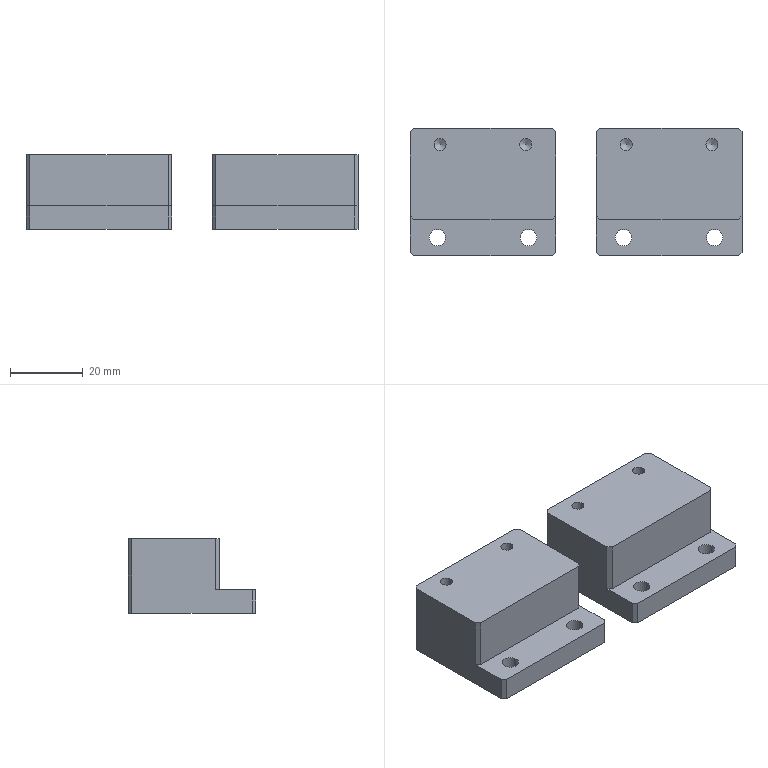Part | NX | 2 solids | 40 faces | box 91 x 35 x 20.5 mm | volume 45300 mm3 | plane 28 | cylinder 8 | cone 4 | commonest cylinder face diameters 3.3 x4 4.5 x4
STEP:
#1=CARTESIAN_POINT('',(-31.,-6.5,-3.75));
#2=VERTEX_POINT('',#1);
#3=CARTESIAN_POINT('',(-32.,-7.5,-3.75));
#4=VERTEX_POINT('',#3);
#5=CARTESIAN_POINT('',(-56.5,-32.,-3.75));
#6=DIRECTION('',(-0.7071,-0.7071,0.));
#7=VECTOR('',#6,1000.);
#8=LINE('',#5,#7);
#9=EDGE_CURVE('',#2,#4,#8,.T.);
#10=ORIENTED_EDGE('',*,*,#9,.F.);
#11=CARTESIAN_POINT('',(-31.,-6.5,10.25));
#12=VERTEX_POINT('',#11);
#13=CARTESIAN_POINT('',(-31.,-6.5,10.25));
#14=DIRECTION('',(0.,0.,-1.));
#15=VECTOR('',#14,1000.);
#16=LINE('',#13,#15);
#17=EDGE_CURVE('',#12,#2,#16,.T.);
#18=ORIENTED_EDGE('',*,*,#17,.F.);
#19=CARTESIAN_POINT('',(-32.,-7.5,10.25));
#20=VERTEX_POINT('',#19);
#21=CARTESIAN_POINT('',(-37.75,-13.25,10.25));
#22=DIRECTION('',(0.7071,0.7071,0.));
#23=VECTOR('',#22,1000.);
#24=LINE('',#21,#23);
#25=EDGE_CURVE('',#20,#12,#24,.T.);
#26=ORIENTED_EDGE('',*,*,#25,.F.);
#27=CARTESIAN_POINT('',(-32.,-7.5,10.25));
#28=DIRECTION('',(0.,0.,1.));
#29=VECTOR('',#28,1000.);
#30=LINE('',#27,#29);
#31=EDGE_CURVE('',#4,#20,#30,.T.);
#32=ORIENTED_EDGE('',*,*,#31,.F.);
#33=EDGE_LOOP('',(#10,#18,#26,#32));
#34=FACE_BOUND('',#33,.T.);
#35=CARTESIAN_POINT('',(-32.,-7.5,10.25));
#36=DIRECTION('',(-0.7071,0.7071,0.));
#37=DIRECTION('',(0.,0.,1.));
#38=AXIS2_PLACEMENT_3D('',#35,#36,#37);
#39=PLANE('',#38);
#40=ADVANCED_FACE('',(#34),#39,.F.);
#41=CARTESIAN_POINT('',(-31.,16.5,10.25));
#42=VERTEX_POINT('',#41);
#43=CARTESIAN_POINT('',(-32.,17.5,10.25));
#44=VERTEX_POINT('',#43);
#45=CARTESIAN_POINT('',(-32.75,18.25,10.25));
#46=DIRECTION('',(-0.7071,0.7071,0.));
#47=VECTOR('',#46,1000.);
#48=LINE('',#45,#47);
#49=EDGE_CURVE('',#42,#44,#48,.T.);
#50=ORIENTED_EDGE('',*,*,#49,.F.);
#51=CARTESIAN_POINT('',(-31.,16.5,-10.25));
#52=VERTEX_POINT('',#51);
#53=CARTESIAN_POINT('',(-31.,16.5,10.25));
#54=DIRECTION('',(0.,0.,1.));
#55=VECTOR('',#54,1000.);
#56=LINE('',#53,#55);
#57=EDGE_CURVE('',#52,#42,#56,.T.);
#58=ORIENTED_EDGE('',*,*,#57,.F.);
#59=CARTESIAN_POINT('',(-32.,17.5,-10.25));
#60=VERTEX_POINT('',#59);
#61=CARTESIAN_POINT('',(-32.,17.5,-10.25));
#62=DIRECTION('',(0.7071,-0.7071,0.));
#63=VECTOR('',#62,1000.);
#64=LINE('',#61,#63);
#65=EDGE_CURVE('',#60,#52,#64,.T.);
#66=ORIENTED_EDGE('',*,*,#65,.F.);
#67=CARTESIAN_POINT('',(-32.,17.5,10.25));
#68=DIRECTION('',(0.,0.,-1.));
#69=VECTOR('',#68,1000.);
#70=LINE('',#67,#69);
#71=EDGE_CURVE('',#44,#60,#70,.T.);
#72=ORIENTED_EDGE('',*,*,#71,.F.);
#73=EDGE_LOOP('',(#50,#58,#66,#72));
#74=FACE_BOUND('',#73,.T.);
#75=CARTESIAN_POINT('',(-32.,17.5,10.25));
#76=DIRECTION('',(-0.7071,-0.7071,0.));
#77=DIRECTION('',(0.,0.,-1.));
#78=AXIS2_PLACEMENT_3D('',#75,#76,#77);
#79=PLANE('',#78);
#80=ADVANCED_FACE('',(#74),#79,.F.);
#81=CARTESIAN_POINT('',(-70.,17.5,10.25));
#82=VERTEX_POINT('',#81);
#83=CARTESIAN_POINT('',(-71.,16.5,10.25));
#84=VERTEX_POINT('',#83);
#85=CARTESIAN_POINT('',(-69.25,18.25,10.25));
#86=DIRECTION('',(-0.7071,-0.7071,0.));
#87=VECTOR('',#86,1000.);
#88=LINE('',#85,#87);
#89=EDGE_CURVE('',#82,#84,#88,.T.);
#90=ORIENTED_EDGE('',*,*,#89,.F.);
#91=CARTESIAN_POINT('',(-70.,17.5,-10.25));
#92=VERTEX_POINT('',#91);
#93=CARTESIAN_POINT('',(-70.,17.5,10.25));
#94=DIRECTION('',(0.,0.,1.));
#95=VECTOR('',#94,1000.);
#96=LINE('',#93,#95);
#97=EDGE_CURVE('',#92,#82,#96,.T.);
#98=ORIENTED_EDGE('',*,*,#97,.F.);
#99=CARTESIAN_POINT('',(-71.,16.5,-10.25));
#100=VERTEX_POINT('',#99);
#101=CARTESIAN_POINT('',(-71.,16.5,-10.25));
#102=DIRECTION('',(0.7071,0.7071,0.));
#103=VECTOR('',#102,1000.);
#104=LINE('',#101,#103);
#105=EDGE_CURVE('',#100,#92,#104,.T.);
#106=ORIENTED_EDGE('',*,*,#105,.F.);
#107=CARTESIAN_POINT('',(-71.,16.5,10.25));
#108=DIRECTION('',(0.,0.,-1.));
#109=VECTOR('',#108,1000.);
#110=LINE('',#107,#109);
#111=EDGE_CURVE('',#84,#100,#110,.T.);
#112=ORIENTED_EDGE('',*,*,#111,.F.);
#113=EDGE_LOOP('',(#90,#98,#106,#112));
#114=FACE_BOUND('',#113,.T.);
#115=CARTESIAN_POINT('',(-71.,16.5,10.25));
#116=DIRECTION('',(0.7071,-0.7071,0.));
#117=DIRECTION('',(0.,0.,-1.));
#118=AXIS2_PLACEMENT_3D('',#115,#116,#117);
#119=PLANE('',#118);
#120=ADVANCED_FACE('',(#114),#119,.F.);
#121=CARTESIAN_POINT('',(-70.,-7.5,-3.75));
#122=VERTEX_POINT('',#121);
#123=CARTESIAN_POINT('',(-71.,-6.5,-3.75));
#124=VERTEX_POINT('',#123);
#125=CARTESIAN_POINT('',(-65.5,-12.,-3.75));
#126=DIRECTION('',(-0.7071,0.7071,0.));
#127=VECTOR('',#126,1000.);
#128=LINE('',#125,#127);
#129=EDGE_CURVE('',#122,#124,#128,.T.);
#130=ORIENTED_EDGE('',*,*,#129,.F.);
#131=CARTESIAN_POINT('',(-70.,-7.5,10.25));
#132=VERTEX_POINT('',#131);
#133=CARTESIAN_POINT('',(-70.,-7.5,10.25));
#134=DIRECTION('',(0.,0.,-1.));
#135=VECTOR('',#134,1000.);
#136=LINE('',#133,#135);
#137=EDGE_CURVE('',#132,#122,#136,.T.);
#138=ORIENTED_EDGE('',*,*,#137,.F.);
#139=CARTESIAN_POINT('',(-71.,-6.5,10.25));
#140=VERTEX_POINT('',#139);
#141=CARTESIAN_POINT('',(-64.25,-13.25,10.25));
#142=DIRECTION('',(0.7071,-0.7071,0.));
#143=VECTOR('',#142,1000.);
#144=LINE('',#141,#143);
#145=EDGE_CURVE('',#140,#132,#144,.T.);
#146=ORIENTED_EDGE('',*,*,#145,.F.);
#147=CARTESIAN_POINT('',(-71.,-6.5,10.25));
#148=DIRECTION('',(0.,0.,1.));
#149=VECTOR('',#148,1000.);
#150=LINE('',#147,#149);
#151=EDGE_CURVE('',#124,#140,#150,.T.);
#152=ORIENTED_EDGE('',*,*,#151,.F.);
#153=EDGE_LOOP('',(#130,#138,#146,#152));
#154=FACE_BOUND('',#153,.T.);
#155=CARTESIAN_POINT('',(-71.,-6.5,10.25));
#156=DIRECTION('',(0.7071,0.7071,0.));
#157=DIRECTION('',(0.,0.,1.));
#158=AXIS2_PLACEMENT_3D('',#155,#156,#157);
#159=PLANE('',#158);
#160=ADVANCED_FACE('',(#154),#159,.F.);
#161=CARTESIAN_POINT('',(-71.,-16.5,-3.75));
#162=VERTEX_POINT('',#161);
#163=CARTESIAN_POINT('',(-70.,-17.5,-3.75));
#164=VERTEX_POINT('',#163);
#165=CARTESIAN_POINT('',(-70.,-17.5,-3.75));
#166=DIRECTION('',(0.7071,-0.7071,0.));
#167=VECTOR('',#166,1000.);
#168=LINE('',#165,#167);
#169=EDGE_CURVE('',#162,#164,#168,.T.);
#170=ORIENTED_EDGE('',*,*,#169,.F.);
#171=CARTESIAN_POINT('',(-71.,-16.5,-10.25));
#172=VERTEX_POINT('',#171);
#173=CARTESIAN_POINT('',(-71.,-16.5,10.25));
#174=DIRECTION('',(0.,0.,1.));
#175=VECTOR('',#174,1000.);
#176=LINE('',#173,#175);
#177=EDGE_CURVE('',#172,#162,#176,.T.);
#178=ORIENTED_EDGE('',*,*,#177,.F.);
#179=CARTESIAN_POINT('',(-70.,-17.5,-10.25));
#180=VERTEX_POINT('',#179);
#181=CARTESIAN_POINT('',(-70.,-17.5,-10.25));
#182=DIRECTION('',(-0.7071,0.7071,0.));
#183=VECTOR('',#182,1000.);
#184=LINE('',#181,#183);
#185=EDGE_CURVE('',#180,#172,#184,.T.);
#186=ORIENTED_EDGE('',*,*,#185,.F.);
#187=CARTESIAN_POINT('',(-70.,-17.5,10.25));
#188=DIRECTION('',(0.,0.,-1.));
#189=VECTOR('',#188,1000.);
#190=LINE('',#187,#189);
#191=EDGE_CURVE('',#164,#180,#190,.T.);
#192=ORIENTED_EDGE('',*,*,#191,.F.);
#193=EDGE_LOOP('',(#170,#178,#186,#192));
#194=FACE_BOUND('',#193,.T.);
#195=CARTESIAN_POINT('',(-70.,-17.5,10.25));
#196=DIRECTION('',(0.7071,0.7071,0.));
#197=DIRECTION('',(0.,0.,-1.));
#198=AXIS2_PLACEMENT_3D('',#195,#196,#197);
#199=PLANE('',#198);
#200=ADVANCED_FACE('',(#194),#199,.F.);
#201=CARTESIAN_POINT('',(-32.,-17.5,-3.75));
#202=VERTEX_POINT('',#201);
#203=CARTESIAN_POINT('',(-31.,-16.5,-3.75));
#204=VERTEX_POINT('',#203);
#205=CARTESIAN_POINT('',(-31.,-16.5,-3.75));
#206=DIRECTION('',(0.7071,0.7071,0.));
#207=VECTOR('',#206,1000.);
#208=LINE('',#205,#207);
#209=EDGE_CURVE('',#202,#204,#208,.T.);
#210=ORIENTED_EDGE('',*,*,#209,.F.);
#211=CARTESIAN_POINT('',(-32.,-17.5,-10.25));
#212=VERTEX_POINT('',#211);
#213=CARTESIAN_POINT('',(-32.,-17.5,10.25));
#214=DIRECTION('',(0.,0.,1.));
#215=VECTOR('',#214,1000.);
#216=LINE('',#213,#215);
#217=EDGE_CURVE('',#212,#202,#216,.T.);
#218=ORIENTED_EDGE('',*,*,#217,.F.);
#219=CARTESIAN_POINT('',(-31.,-16.5,-10.25));
#220=VERTEX_POINT('',#219);
#221=CARTESIAN_POINT('',(-31.,-16.5,-10.25));
#222=DIRECTION('',(-0.7071,-0.7071,0.));
#223=VECTOR('',#222,1000.);
#224=LINE('',#221,#223);
#225=EDGE_CURVE('',#220,#212,#224,.T.);
#226=ORIENTED_EDGE('',*,*,#225,.F.);
#227=CARTESIAN_POINT('',(-31.,-16.5,10.25));
#228=DIRECTION('',(0.,0.,-1.));
#229=VECTOR('',#228,1000.);
#230=LINE('',#227,#229);
#231=EDGE_CURVE('',#204,#220,#230,.T.);
#232=ORIENTED_EDGE('',*,*,#231,.F.);
#233=EDGE_LOOP('',(#210,#218,#226,#232));
#234=FACE_BOUND('',#233,.T.);
#235=CARTESIAN_POINT('',(-31.,-16.5,10.25));
#236=DIRECTION('',(-0.7071,0.7071,0.));
#237=DIRECTION('',(0.,0.,-1.));
#238=AXIS2_PLACEMENT_3D('',#235,#236,#237);
#239=PLANE('',#238);
#240=ADVANCED_FACE('',(#234),#239,.F.);
#241=CARTESIAN_POINT('',(-71.,-17.5,-3.75));
#242=DIRECTION('',(1.,0.,0.));
#243=VECTOR('',#242,1000.);
#244=LINE('',#241,#243);
#245=EDGE_CURVE('',#164,#202,#244,.T.);
#246=ORIENTED_EDGE('',*,*,#245,.T.);
#247=ORIENTED_EDGE('',*,*,#209,.T.);
#248=CARTESIAN_POINT('',(-31.,-17.5,-3.75));
#249=DIRECTION('',(0.,1.,0.));
#250=VECTOR('',#249,1000.);
#251=LINE('',#248,#250);
#252=EDGE_CURVE('',#204,#2,#251,.T.);
#253=ORIENTED_EDGE('',*,*,#252,.T.);
#254=ORIENTED_EDGE('',*,*,#9,.T.);
#255=CARTESIAN_POINT('',(-71.,-7.5,-3.75));
#256=DIRECTION('',(1.,0.,0.));
#257=VECTOR('',#256,1000.);
#258=LINE('',#255,#257);
#259=EDGE_CURVE('',#122,#4,#258,.T.);
#260=ORIENTED_EDGE('',*,*,#259,.F.);
#261=ORIENTED_EDGE('',*,*,#129,.T.);
#262=CARTESIAN_POINT('',(-71.,-17.5,-3.75));
#263=DIRECTION('',(0.,1.,0.));
#264=VECTOR('',#263,1000.);
#265=LINE('',#262,#264);
#266=EDGE_CURVE('',#162,#124,#265,.T.);
#267=ORIENTED_EDGE('',*,*,#266,.F.);
#268=ORIENTED_EDGE('',*,*,#169,.T.);
#269=EDGE_LOOP('',(#246,#247,#253,#254,#260,#261,#267,#268));
#270=FACE_BOUND('',#269,.T.);
#271=CARTESIAN_POINT('',(-36.25,-12.5,-3.75));
#272=VERTEX_POINT('',#271);
#273=CARTESIAN_POINT('',(-38.5,-12.5,-3.75));
#274=DIRECTION('',(0.,0.,1.));
#275=DIRECTION('',(1.,0.,0.));
#276=AXIS2_PLACEMENT_3D('',#273,#274,#275);
#277=CIRCLE('',#276,2.25);
#278=EDGE_CURVE('',#272,#272,#277,.T.);
#279=ORIENTED_EDGE('',*,*,#278,.F.);
#280=EDGE_LOOP('',(#279));
#281=FACE_BOUND('',#280,.T.);
#282=CARTESIAN_POINT('',(-61.25,-12.5,-3.75));
#283=VERTEX_POINT('',#282);
#284=CARTESIAN_POINT('',(-63.5,-12.5,-3.75));
#285=DIRECTION('',(0.,0.,1.));
#286=DIRECTION('',(1.,0.,0.));
#287=AXIS2_PLACEMENT_3D('',#284,#285,#286);
#288=CIRCLE('',#287,2.25);
#289=EDGE_CURVE('',#283,#283,#288,.T.);
#290=ORIENTED_EDGE('',*,*,#289,.F.);
#291=EDGE_LOOP('',(#290));
#292=FACE_BOUND('',#291,.T.);
#293=CARTESIAN_POINT('',(-71.,-17.5,-3.75));
#294=DIRECTION('',(0.,0.,-1.));
#295=DIRECTION('',(-1.,0.,0.));
#296=AXIS2_PLACEMENT_3D('',#293,#294,#295);
#297=PLANE('',#296);
#298=ADVANCED_FACE('',(#270,#281,#292),#297,.F.);
#299=CARTESIAN_POINT('',(-71.,-7.5,10.25));
#300=DIRECTION('',(1.,0.,0.));
#301=VECTOR('',#300,1000.);
#302=LINE('',#299,#301);
#303=EDGE_CURVE('',#132,#20,#302,.T.);
#304=ORIENTED_EDGE('',*,*,#303,.F.);
#305=ORIENTED_EDGE('',*,*,#137,.T.);
#306=ORIENTED_EDGE('',*,*,#259,.T.);
#307=ORIENTED_EDGE('',*,*,#31,.T.);
#308=EDGE_LOOP('',(#304,#305,#306,#307));
#309=FACE_BOUND('',#308,.T.);
#310=CARTESIAN_POINT('',(-71.,-7.5,10.25));
#311=DIRECTION('',(0.,1.,0.));
#312=DIRECTION('',(-1.,0.,0.));
#313=AXIS2_PLACEMENT_3D('',#310,#311,#312);
#314=PLANE('',#313);
#315=ADVANCED_FACE('',(#309),#314,.F.);
#316=CARTESIAN_POINT('',(-31.,17.5,-10.25));
#317=DIRECTION('',(0.,1.,0.));
#318=VECTOR('',#317,1000.);
#319=LINE('',#316,#318);
#320=EDGE_CURVE('',#220,#52,#319,.T.);
#321=ORIENTED_EDGE('',*,*,#320,.F.);
#322=ORIENTED_EDGE('',*,*,#225,.T.);
#323=CARTESIAN_POINT('',(-71.,-17.5,-10.25));
#324=DIRECTION('',(1.,0.,0.));
#325=VECTOR('',#324,1000.);
#326=LINE('',#323,#325);
#327=EDGE_CURVE('',#180,#212,#326,.T.);
#328=ORIENTED_EDGE('',*,*,#327,.F.);
#329=ORIENTED_EDGE('',*,*,#185,.T.);
#330=CARTESIAN_POINT('',(-71.,17.5,-10.25));
#331=DIRECTION('',(0.,-1.,0.));
#332=VECTOR('',#331,1000.);
#333=LINE('',#330,#332);
#334=EDGE_CURVE('',#100,#172,#333,.T.);
#335=ORIENTED_EDGE('',*,*,#334,.F.);
#336=ORIENTED_EDGE('',*,*,#105,.T.);
#337=CARTESIAN_POINT('',(-71.,17.5,-10.25));
#338=DIRECTION('',(-1.,0.,0.));
#339=VECTOR('',#338,1000.);
#340=LINE('',#337,#339);
#341=EDGE_CURVE('',#60,#92,#340,.T.);
#342=ORIENTED_EDGE('',*,*,#341,.F.);
#343=ORIENTED_EDGE('',*,*,#65,.T.);
#344=EDGE_LOOP('',(#321,#322,#328,#329,#335,#336,#342,#343));
#345=FACE_BOUND('',#344,.T.);
#346=CARTESIAN_POINT('',(-36.25,-12.5,-10.25));
#347=VERTEX_POINT('',#346);
#348=CARTESIAN_POINT('',(-38.5,-12.5,-10.25));
#349=DIRECTION('',(0.,0.,1.));
#350=DIRECTION('',(1.,0.,0.));
#351=AXIS2_PLACEMENT_3D('',#348,#349,#350);
#352=CIRCLE('',#351,2.25);
#353=EDGE_CURVE('',#347,#347,#352,.T.);
#354=ORIENTED_EDGE('',*,*,#353,.T.);
#355=EDGE_LOOP('',(#354));
#356=FACE_BOUND('',#355,.T.);
#357=CARTESIAN_POINT('',(-61.25,-12.5,-10.25));
#358=VERTEX_POINT('',#357);
#359=CARTESIAN_POINT('',(-63.5,-12.5,-10.25));
#360=DIRECTION('',(0.,0.,1.));
#361=DIRECTION('',(1.,0.,0.));
#362=AXIS2_PLACEMENT_3D('',#359,#360,#361);
#363=CIRCLE('',#362,2.25);
#364=EDGE_CURVE('',#358,#358,#363,.T.);
#365=ORIENTED_EDGE('',*,*,#364,.T.);
#366=EDGE_LOOP('',(#365));
#367=FACE_BOUND('',#366,.T.);
#368=CARTESIAN_POINT('',(-51.,0.,-10.25));
#369=DIRECTION('',(0.,0.,1.));
#370=DIRECTION('',(1.,0.,0.));
#371=AXIS2_PLACEMENT_3D('',#368,#369,#370);
#372=PLANE('',#371);
#373=ADVANCED_FACE('',(#345,#356,#367),#372,.F.);
#374=CARTESIAN_POINT('',(-71.,17.5,10.25));
#375=DIRECTION('',(0.,-1.,0.));
#376=VECTOR('',#375,1000.);
#377=LINE('',#374,#376);
#378=EDGE_CURVE('',#84,#140,#377,.T.);
#379=ORIENTED_EDGE('',*,*,#378,.T.);
#380=ORIENTED_EDGE('',*,*,#145,.T.);
#381=ORIENTED_EDGE('',*,*,#303,.T.);
#382=ORIENTED_EDGE('',*,*,#25,.T.);
#383=CARTESIAN_POINT('',(-31.,17.5,10.25));
#384=DIRECTION('',(0.,1.,0.));
#385=VECTOR('',#384,1000.);
#386=LINE('',#383,#385);
#387=EDGE_CURVE('',#12,#42,#386,.T.);
#388=ORIENTED_EDGE('',*,*,#387,.T.);
#389=ORIENTED_EDGE('',*,*,#49,.T.);
#390=CARTESIAN_POINT('',(-71.,17.5,10.25));
#391=DIRECTION('',(-1.,0.,0.));
#392=VECTOR('',#391,1000.);
#393=LINE('',#390,#392);
#394=EDGE_CURVE('',#44,#82,#393,.T.);
#395=ORIENTED_EDGE('',*,*,#394,.T.);
#396=ORIENTED_EDGE('',*,*,#89,.T.);
#397=EDGE_LOOP('',(#379,#380,#381,#382,#388,#389,#395,#396));
#398=FACE_BOUND('',#397,.T.);
#399=CARTESIAN_POINT('',(-37.6,13.,10.25));
#400=VERTEX_POINT('',#399);
#401=CARTESIAN_POINT('',(-39.25,13.,10.25));
#402=DIRECTION('',(0.,0.,1.));
#403=DIRECTION('',(1.,0.,0.));
#404=AXIS2_PLACEMENT_3D('',#401,#402,#403);
#405=CIRCLE('',#404,1.65);
#406=EDGE_CURVE('',#400,#400,#405,.T.);
#407=ORIENTED_EDGE('',*,*,#406,.F.);
#408=EDGE_LOOP('',(#407));
#409=FACE_BOUND('',#408,.T.);
#410=CARTESIAN_POINT('',(-61.1,13.,10.25));
#411=VERTEX_POINT('',#410);
#412=CARTESIAN_POINT('',(-62.75,13.,10.25));
#413=DIRECTION('',(0.,0.,1.));
#414=DIRECTION('',(1.,0.,0.));
#415=AXIS2_PLACEMENT_3D('',#412,#413,#414);
#416=CIRCLE('',#415,1.65);
#417=EDGE_CURVE('',#411,#411,#416,.T.);
#418=ORIENTED_EDGE('',*,*,#417,.F.);
#419=EDGE_LOOP('',(#418));
#420=FACE_BOUND('',#419,.T.);
#421=CARTESIAN_POINT('',(-51.,0.,10.25));
#422=DIRECTION('',(0.,0.,1.));
#423=DIRECTION('',(1.,0.,0.));
#424=AXIS2_PLACEMENT_3D('',#421,#422,#423);
#425=PLANE('',#424);
#426=ADVANCED_FACE('',(#398,#409,#420),#425,.T.);
#427=ORIENTED_EDGE('',*,*,#327,.T.);
#428=ORIENTED_EDGE('',*,*,#217,.T.);
#429=ORIENTED_EDGE('',*,*,#245,.F.);
#430=ORIENTED_EDGE('',*,*,#191,.T.);
#431=EDGE_LOOP('',(#427,#428,#429,#430));
#432=FACE_BOUND('',#431,.T.);
#433=CARTESIAN_POINT('',(-71.,-17.5,10.25));
#434=DIRECTION('',(0.,1.,0.));
#435=DIRECTION('',(0.,0.,1.));
#436=AXIS2_PLACEMENT_3D('',#433,#434,#435);
#437=PLANE('',#436);
#438=ADVANCED_FACE('',(#432),#437,.F.);
#439=ORIENTED_EDGE('',*,*,#334,.T.);
#440=ORIENTED_EDGE('',*,*,#177,.T.);
#441=ORIENTED_EDGE('',*,*,#266,.T.);
#442=ORIENTED_EDGE('',*,*,#151,.T.);
#443=ORIENTED_EDGE('',*,*,#378,.F.);
#444=ORIENTED_EDGE('',*,*,#111,.T.);
#445=EDGE_LOOP('',(#439,#440,#441,#442,#443,#444));
#446=FACE_BOUND('',#445,.T.);
#447=CARTESIAN_POINT('',(-71.,17.5,10.25));
#448=DIRECTION('',(1.,0.,0.));
#449=DIRECTION('',(0.,1.,0.));
#450=AXIS2_PLACEMENT_3D('',#447,#448,#449);
#451=PLANE('',#450);
#452=ADVANCED_FACE('',(#446),#451,.F.);
#453=ORIENTED_EDGE('',*,*,#341,.T.);
#454=ORIENTED_EDGE('',*,*,#97,.T.);
#455=ORIENTED_EDGE('',*,*,#394,.F.);
#456=ORIENTED_EDGE('',*,*,#71,.T.);
#457=EDGE_LOOP('',(#453,#454,#455,#456));
#458=FACE_BOUND('',#457,.T.);
#459=CARTESIAN_POINT('',(-71.,17.5,10.25));
#460=DIRECTION('',(0.,-1.,0.));
#461=DIRECTION('',(0.,0.,-1.));
#462=AXIS2_PLACEMENT_3D('',#459,#460,#461);
#463=PLANE('',#462);
#464=ADVANCED_FACE('',(#458),#463,.F.);
#465=ORIENTED_EDGE('',*,*,#252,.F.);
#466=ORIENTED_EDGE('',*,*,#231,.T.);
#467=ORIENTED_EDGE('',*,*,#320,.T.);
#468=ORIENTED_EDGE('',*,*,#57,.T.);
#469=ORIENTED_EDGE('',*,*,#387,.F.);
#470=ORIENTED_EDGE('',*,*,#17,.T.);
#471=EDGE_LOOP('',(#465,#466,#467,#468,#469,#470));
#472=FACE_BOUND('',#471,.T.);
#473=CARTESIAN_POINT('',(-31.,17.5,10.25));
#474=DIRECTION('',(-1.,0.,0.));
#475=DIRECTION('',(0.,-1.,0.));
#476=AXIS2_PLACEMENT_3D('',#473,#474,#475);
#477=PLANE('',#476);
#478=ADVANCED_FACE('',(#472),#477,.F.);
#479=CARTESIAN_POINT('',(-37.6,13.,-1.25));
#480=VERTEX_POINT('',#479);
#481=CARTESIAN_POINT('',(-39.25,13.,-1.25));
#482=DIRECTION('',(0.,0.,1.));
#483=DIRECTION('',(1.,0.,0.));
#484=AXIS2_PLACEMENT_3D('',#481,#482,#483);
#485=CIRCLE('',#484,1.65);
#486=EDGE_CURVE('',#480,#480,#485,.T.);
#487=ORIENTED_EDGE('',*,*,#486,.T.);
#488=EDGE_LOOP('',(#487));
#489=FACE_BOUND('',#488,.T.);
#490=CARTESIAN_POINT('',(-39.25,13.,-2.241));
#491=VERTEX_POINT('',#490);
#492=VERTEX_LOOP('',#491);
#493=FACE_BOUND('',#492,.T.);
#494=CARTESIAN_POINT('',(-39.25,13.,-1.25));
#495=DIRECTION('',(0.,0.,1.));
#496=DIRECTION('',(1.,0.,0.));
#497=AXIS2_PLACEMENT_3D('',#494,#495,#496);
#498=CONICAL_SURFACE('',#497,1.65,1.03);
#499=ADVANCED_FACE('',(#489,#493),#498,.F.);
#500=ORIENTED_EDGE('',*,*,#486,.F.);
#501=EDGE_LOOP('',(#500));
#502=FACE_BOUND('',#501,.T.);
#503=ORIENTED_EDGE('',*,*,#406,.T.);
#504=EDGE_LOOP('',(#503));
#505=FACE_BOUND('',#504,.T.);
#506=CARTESIAN_POINT('',(-39.25,13.,10.25));
#507=DIRECTION('',(0.,0.,1.));
#508=DIRECTION('',(1.,0.,0.));
#509=AXIS2_PLACEMENT_3D('',#506,#507,#508);
#510=CYLINDRICAL_SURFACE('',#509,1.65);
#511=ADVANCED_FACE('',(#502,#505),#510,.F.);
#512=CARTESIAN_POINT('',(-61.1,13.,-1.25));
#513=VERTEX_POINT('',#512);
#514=CARTESIAN_POINT('',(-62.75,13.,-1.25));
#515=DIRECTION('',(0.,0.,1.));
#516=DIRECTION('',(1.,0.,0.));
#517=AXIS2_PLACEMENT_3D('',#514,#515,#516);
#518=CIRCLE('',#517,1.65);
#519=EDGE_CURVE('',#513,#513,#518,.T.);
#520=ORIENTED_EDGE('',*,*,#519,.T.);
#521=EDGE_LOOP('',(#520));
#522=FACE_BOUND('',#521,.T.);
#523=CARTESIAN_POINT('',(-62.75,13.,-2.241));
#524=VERTEX_POINT('',#523);
#525=VERTEX_LOOP('',#524);
#526=FACE_BOUND('',#525,.T.);
#527=CARTESIAN_POINT('',(-62.75,13.,-1.25));
#528=DIRECTION('',(0.,0.,1.));
#529=DIRECTION('',(1.,0.,0.));
#530=AXIS2_PLACEMENT_3D('',#527,#528,#529);
#531=CONICAL_SURFACE('',#530,1.65,1.03);
#532=ADVANCED_FACE('',(#522,#526),#531,.F.);
#533=ORIENTED_EDGE('',*,*,#519,.F.);
#534=EDGE_LOOP('',(#533));
#535=FACE_BOUND('',#534,.T.);
#536=ORIENTED_EDGE('',*,*,#417,.T.);
#537=EDGE_LOOP('',(#536));
#538=FACE_BOUND('',#537,.T.);
#539=CARTESIAN_POINT('',(-62.75,13.,10.25));
#540=DIRECTION('',(0.,0.,1.));
#541=DIRECTION('',(1.,0.,0.));
#542=AXIS2_PLACEMENT_3D('',#539,#540,#541);
#543=CYLINDRICAL_SURFACE('',#542,1.65);
#544=ADVANCED_FACE('',(#535,#538),#543,.F.);
#545=ORIENTED_EDGE('',*,*,#353,.F.);
#546=EDGE_LOOP('',(#545));
#547=FACE_BOUND('',#546,.T.);
#548=ORIENTED_EDGE('',*,*,#278,.T.);
#549=EDGE_LOOP('',(#548));
#550=FACE_BOUND('',#549,.T.);
#551=CARTESIAN_POINT('',(-38.5,-12.5,-3.75));
#552=DIRECTION('',(0.,0.,1.));
#553=DIRECTION('',(1.,0.,0.));
#554=AXIS2_PLACEMENT_3D('',#551,#552,#553);
#555=CYLINDRICAL_SURFACE('',#554,2.25);
#556=ADVANCED_FACE('',(#547,#550),#555,.F.);
#557=ORIENTED_EDGE('',*,*,#364,.F.);
#558=EDGE_LOOP('',(#557));
#559=FACE_BOUND('',#558,.T.);
#560=ORIENTED_EDGE('',*,*,#289,.T.);
#561=EDGE_LOOP('',(#560));
#562=FACE_BOUND('',#561,.T.);
#563=CARTESIAN_POINT('',(-63.5,-12.5,-3.75));
#564=DIRECTION('',(0.,0.,1.));
#565=DIRECTION('',(1.,0.,0.));
#566=AXIS2_PLACEMENT_3D('',#563,#564,#565);
#567=CYLINDRICAL_SURFACE('',#566,2.25);
#568=ADVANCED_FACE('',(#559,#562),#567,.F.);
#569=CLOSED_SHELL('',(#40,#80,#120,#160,#200,#240,#298,#315,#373,#426,#438,#452,#464,#478,#499,#511,#532,#544,#556,#568));
#570=MANIFOLD_SOLID_BREP('',#569);
#571=CARTESIAN_POINT('',(20.,-6.5,-3.75));
#572=VERTEX_POINT('',#571);
#573=CARTESIAN_POINT('',(19.,-7.5,-3.75));
#574=VERTEX_POINT('',#573);
#575=CARTESIAN_POINT('',(-5.5,-32.,-3.75));
#576=DIRECTION('',(-0.7071,-0.7071,0.));
#577=VECTOR('',#576,1000.);
#578=LINE('',#575,#577);
#579=EDGE_CURVE('',#572,#574,#578,.T.);
#580=ORIENTED_EDGE('',*,*,#579,.F.);
#581=CARTESIAN_POINT('',(20.,-6.5,10.25));
#582=VERTEX_POINT('',#581);
#583=CARTESIAN_POINT('',(20.,-6.5,10.25));
#584=DIRECTION('',(0.,0.,-1.));
#585=VECTOR('',#584,1000.);
#586=LINE('',#583,#585);
#587=EDGE_CURVE('',#582,#572,#586,.T.);
#588=ORIENTED_EDGE('',*,*,#587,.F.);
#589=CARTESIAN_POINT('',(19.,-7.5,10.25));
#590=VERTEX_POINT('',#589);
#591=CARTESIAN_POINT('',(13.25,-13.25,10.25));
#592=DIRECTION('',(0.7071,0.7071,0.));
#593=VECTOR('',#592,1000.);
#594=LINE('',#591,#593);
#595=EDGE_CURVE('',#590,#582,#594,.T.);
#596=ORIENTED_EDGE('',*,*,#595,.F.);
#597=CARTESIAN_POINT('',(19.,-7.5,10.25));
#598=DIRECTION('',(0.,0.,1.));
#599=VECTOR('',#598,1000.);
#600=LINE('',#597,#599);
#601=EDGE_CURVE('',#574,#590,#600,.T.);
#602=ORIENTED_EDGE('',*,*,#601,.F.);
#603=EDGE_LOOP('',(#580,#588,#596,#602));
#604=FACE_BOUND('',#603,.T.);
#605=CARTESIAN_POINT('',(19.,-7.5,10.25));
#606=DIRECTION('',(-0.7071,0.7071,0.));
#607=DIRECTION('',(0.,0.,1.));
#608=AXIS2_PLACEMENT_3D('',#605,#606,#607);
#609=PLANE('',#608);
#610=ADVANCED_FACE('',(#604),#609,.F.);
#611=CARTESIAN_POINT('',(20.,16.5,10.25));
#612=VERTEX_POINT('',#611);
#613=CARTESIAN_POINT('',(19.,17.5,10.25));
#614=VERTEX_POINT('',#613);
#615=CARTESIAN_POINT('',(18.25,18.25,10.25));
#616=DIRECTION('',(-0.7071,0.7071,0.));
#617=VECTOR('',#616,1000.);
#618=LINE('',#615,#617);
#619=EDGE_CURVE('',#612,#614,#618,.T.);
#620=ORIENTED_EDGE('',*,*,#619,.F.);
#621=CARTESIAN_POINT('',(20.,16.5,-10.25));
#622=VERTEX_POINT('',#621);
#623=CARTESIAN_POINT('',(20.,16.5,10.25));
#624=DIRECTION('',(0.,0.,1.));
#625=VECTOR('',#624,1000.);
#626=LINE('',#623,#625);
#627=EDGE_CURVE('',#622,#612,#626,.T.);
#628=ORIENTED_EDGE('',*,*,#627,.F.);
#629=CARTESIAN_POINT('',(19.,17.5,-10.25));
#630=VERTEX_POINT('',#629);
#631=CARTESIAN_POINT('',(19.,17.5,-10.25));
#632=DIRECTION('',(0.7071,-0.7071,0.));
#633=VECTOR('',#632,1000.);
#634=LINE('',#631,#633);
#635=EDGE_CURVE('',#630,#622,#634,.T.);
#636=ORIENTED_EDGE('',*,*,#635,.F.);
#637=CARTESIAN_POINT('',(19.,17.5,10.25));
#638=DIRECTION('',(0.,0.,-1.));
#639=VECTOR('',#638,1000.);
#640=LINE('',#637,#639);
#641=EDGE_CURVE('',#614,#630,#640,.T.);
#642=ORIENTED_EDGE('',*,*,#641,.F.);
#643=EDGE_LOOP('',(#620,#628,#636,#642));
#644=FACE_BOUND('',#643,.T.);
#645=CARTESIAN_POINT('',(19.,17.5,10.25));
#646=DIRECTION('',(-0.7071,-0.7071,0.));
#647=DIRECTION('',(0.,0.,-1.));
#648=AXIS2_PLACEMENT_3D('',#645,#646,#647);
#649=PLANE('',#648);
#650=ADVANCED_FACE('',(#644),#649,.F.);
#651=CARTESIAN_POINT('',(-19.,17.5,10.25));
#652=VERTEX_POINT('',#651);
#653=CARTESIAN_POINT('',(-20.,16.5,10.25));
#654=VERTEX_POINT('',#653);
#655=CARTESIAN_POINT('',(-18.25,18.25,10.25));
#656=DIRECTION('',(-0.7071,-0.7071,0.));
#657=VECTOR('',#656,1000.);
#658=LINE('',#655,#657);
#659=EDGE_CURVE('',#652,#654,#658,.T.);
#660=ORIENTED_EDGE('',*,*,#659,.F.);
#661=CARTESIAN_POINT('',(-19.,17.5,-10.25));
#662=VERTEX_POINT('',#661);
#663=CARTESIAN_POINT('',(-19.,17.5,10.25));
#664=DIRECTION('',(0.,0.,1.));
#665=VECTOR('',#664,1000.);
#666=LINE('',#663,#665);
#667=EDGE_CURVE('',#662,#652,#666,.T.);
#668=ORIENTED_EDGE('',*,*,#667,.F.);
#669=CARTESIAN_POINT('',(-20.,16.5,-10.25));
#670=VERTEX_POINT('',#669);
#671=CARTESIAN_POINT('',(-20.,16.5,-10.25));
#672=DIRECTION('',(0.7071,0.7071,0.));
#673=VECTOR('',#672,1000.);
#674=LINE('',#671,#673);
#675=EDGE_CURVE('',#670,#662,#674,.T.);
#676=ORIENTED_EDGE('',*,*,#675,.F.);
#677=CARTESIAN_POINT('',(-20.,16.5,10.25));
#678=DIRECTION('',(0.,0.,-1.));
#679=VECTOR('',#678,1000.);
#680=LINE('',#677,#679);
#681=EDGE_CURVE('',#654,#670,#680,.T.);
#682=ORIENTED_EDGE('',*,*,#681,.F.);
#683=EDGE_LOOP('',(#660,#668,#676,#682));
#684=FACE_BOUND('',#683,.T.);
#685=CARTESIAN_POINT('',(-20.,16.5,10.25));
#686=DIRECTION('',(0.7071,-0.7071,0.));
#687=DIRECTION('',(0.,0.,-1.));
#688=AXIS2_PLACEMENT_3D('',#685,#686,#687);
#689=PLANE('',#688);
#690=ADVANCED_FACE('',(#684),#689,.F.);
#691=CARTESIAN_POINT('',(-19.,-7.5,-3.75));
#692=VERTEX_POINT('',#691);
#693=CARTESIAN_POINT('',(-20.,-6.5,-3.75));
#694=VERTEX_POINT('',#693);
#695=CARTESIAN_POINT('',(-14.5,-12.,-3.75));
#696=DIRECTION('',(-0.7071,0.7071,0.));
#697=VECTOR('',#696,1000.);
#698=LINE('',#695,#697);
#699=EDGE_CURVE('',#692,#694,#698,.T.);
#700=ORIENTED_EDGE('',*,*,#699,.F.);
#701=CARTESIAN_POINT('',(-19.,-7.5,10.25));
#702=VERTEX_POINT('',#701);
#703=CARTESIAN_POINT('',(-19.,-7.5,10.25));
#704=DIRECTION('',(0.,0.,-1.));
#705=VECTOR('',#704,1000.);
#706=LINE('',#703,#705);
#707=EDGE_CURVE('',#702,#692,#706,.T.);
#708=ORIENTED_EDGE('',*,*,#707,.F.);
#709=CARTESIAN_POINT('',(-20.,-6.5,10.25));
#710=VERTEX_POINT('',#709);
#711=CARTESIAN_POINT('',(-13.25,-13.25,10.25));
#712=DIRECTION('',(0.7071,-0.7071,0.));
#713=VECTOR('',#712,1000.);
#714=LINE('',#711,#713);
#715=EDGE_CURVE('',#710,#702,#714,.T.);
#716=ORIENTED_EDGE('',*,*,#715,.F.);
#717=CARTESIAN_POINT('',(-20.,-6.5,10.25));
#718=DIRECTION('',(0.,0.,1.));
#719=VECTOR('',#718,1000.);
#720=LINE('',#717,#719);
#721=EDGE_CURVE('',#694,#710,#720,.T.);
#722=ORIENTED_EDGE('',*,*,#721,.F.);
#723=EDGE_LOOP('',(#700,#708,#716,#722));
#724=FACE_BOUND('',#723,.T.);
#725=CARTESIAN_POINT('',(-20.,-6.5,10.25));
#726=DIRECTION('',(0.7071,0.7071,0.));
#727=DIRECTION('',(0.,0.,1.));
#728=AXIS2_PLACEMENT_3D('',#725,#726,#727);
#729=PLANE('',#728);
#730=ADVANCED_FACE('',(#724),#729,.F.);
#731=CARTESIAN_POINT('',(-20.,-16.5,-3.75));
#732=VERTEX_POINT('',#731);
#733=CARTESIAN_POINT('',(-19.,-17.5,-3.75));
#734=VERTEX_POINT('',#733);
#735=CARTESIAN_POINT('',(-19.,-17.5,-3.75));
#736=DIRECTION('',(0.7071,-0.7071,0.));
#737=VECTOR('',#736,1000.);
#738=LINE('',#735,#737);
#739=EDGE_CURVE('',#732,#734,#738,.T.);
#740=ORIENTED_EDGE('',*,*,#739,.F.);
#741=CARTESIAN_POINT('',(-20.,-16.5,-10.25));
#742=VERTEX_POINT('',#741);
#743=CARTESIAN_POINT('',(-20.,-16.5,10.25));
#744=DIRECTION('',(0.,0.,1.));
#745=VECTOR('',#744,1000.);
#746=LINE('',#743,#745);
#747=EDGE_CURVE('',#742,#732,#746,.T.);
#748=ORIENTED_EDGE('',*,*,#747,.F.);
#749=CARTESIAN_POINT('',(-19.,-17.5,-10.25));
#750=VERTEX_POINT('',#749);
#751=CARTESIAN_POINT('',(-19.,-17.5,-10.25));
#752=DIRECTION('',(-0.7071,0.7071,0.));
#753=VECTOR('',#752,1000.);
#754=LINE('',#751,#753);
#755=EDGE_CURVE('',#750,#742,#754,.T.);
#756=ORIENTED_EDGE('',*,*,#755,.F.);
#757=CARTESIAN_POINT('',(-19.,-17.5,10.25));
#758=DIRECTION('',(0.,0.,-1.));
#759=VECTOR('',#758,1000.);
#760=LINE('',#757,#759);
#761=EDGE_CURVE('',#734,#750,#760,.T.);
#762=ORIENTED_EDGE('',*,*,#761,.F.);
#763=EDGE_LOOP('',(#740,#748,#756,#762));
#764=FACE_BOUND('',#763,.T.);
#765=CARTESIAN_POINT('',(-19.,-17.5,10.25));
#766=DIRECTION('',(0.7071,0.7071,0.));
#767=DIRECTION('',(0.,0.,-1.));
#768=AXIS2_PLACEMENT_3D('',#765,#766,#767);
#769=PLANE('',#768);
#770=ADVANCED_FACE('',(#764),#769,.F.);
#771=CARTESIAN_POINT('',(19.,-17.5,-3.75));
#772=VERTEX_POINT('',#771);
#773=CARTESIAN_POINT('',(20.,-16.5,-3.75));
#774=VERTEX_POINT('',#773);
#775=CARTESIAN_POINT('',(20.,-16.5,-3.75));
#776=DIRECTION('',(0.7071,0.7071,0.));
#777=VECTOR('',#776,1000.);
#778=LINE('',#775,#777);
#779=EDGE_CURVE('',#772,#774,#778,.T.);
#780=ORIENTED_EDGE('',*,*,#779,.F.);
#781=CARTESIAN_POINT('',(19.,-17.5,-10.25));
#782=VERTEX_POINT('',#781);
#783=CARTESIAN_POINT('',(19.,-17.5,10.25));
#784=DIRECTION('',(0.,0.,1.));
#785=VECTOR('',#784,1000.);
#786=LINE('',#783,#785);
#787=EDGE_CURVE('',#782,#772,#786,.T.);
#788=ORIENTED_EDGE('',*,*,#787,.F.);
#789=CARTESIAN_POINT('',(20.,-16.5,-10.25));
#790=VERTEX_POINT('',#789);
#791=CARTESIAN_POINT('',(20.,-16.5,-10.25));
#792=DIRECTION('',(-0.7071,-0.7071,0.));
#793=VECTOR('',#792,1000.);
#794=LINE('',#791,#793);
#795=EDGE_CURVE('',#790,#782,#794,.T.);
#796=ORIENTED_EDGE('',*,*,#795,.F.);
#797=CARTESIAN_POINT('',(20.,-16.5,10.25));
#798=DIRECTION('',(0.,0.,-1.));
#799=VECTOR('',#798,1000.);
#800=LINE('',#797,#799);
#801=EDGE_CURVE('',#774,#790,#800,.T.);
#802=ORIENTED_EDGE('',*,*,#801,.F.);
#803=EDGE_LOOP('',(#780,#788,#796,#802));
#804=FACE_BOUND('',#803,.T.);
#805=CARTESIAN_POINT('',(20.,-16.5,10.25));
#806=DIRECTION('',(-0.7071,0.7071,0.));
#807=DIRECTION('',(0.,0.,-1.));
#808=AXIS2_PLACEMENT_3D('',#805,#806,#807);
#809=PLANE('',#808);
#810=ADVANCED_FACE('',(#804),#809,.F.);
#811=CARTESIAN_POINT('',(-20.,-17.5,-3.75));
#812=DIRECTION('',(1.,0.,0.));
#813=VECTOR('',#812,1000.);
#814=LINE('',#811,#813);
#815=EDGE_CURVE('',#734,#772,#814,.T.);
#816=ORIENTED_EDGE('',*,*,#815,.T.);
#817=ORIENTED_EDGE('',*,*,#779,.T.);
#818=CARTESIAN_POINT('',(20.,-17.5,-3.75));
#819=DIRECTION('',(0.,1.,0.));
#820=VECTOR('',#819,1000.);
#821=LINE('',#818,#820);
#822=EDGE_CURVE('',#774,#572,#821,.T.);
#823=ORIENTED_EDGE('',*,*,#822,.T.);
#824=ORIENTED_EDGE('',*,*,#579,.T.);
#825=CARTESIAN_POINT('',(-20.,-7.5,-3.75));
#826=DIRECTION('',(1.,0.,0.));
#827=VECTOR('',#826,1000.);
#828=LINE('',#825,#827);
#829=EDGE_CURVE('',#692,#574,#828,.T.);
#830=ORIENTED_EDGE('',*,*,#829,.F.);
#831=ORIENTED_EDGE('',*,*,#699,.T.);
#832=CARTESIAN_POINT('',(-20.,-17.5,-3.75));
#833=DIRECTION('',(0.,1.,0.));
#834=VECTOR('',#833,1000.);
#835=LINE('',#832,#834);
#836=EDGE_CURVE('',#732,#694,#835,.T.);
#837=ORIENTED_EDGE('',*,*,#836,.F.);
#838=ORIENTED_EDGE('',*,*,#739,.T.);
#839=EDGE_LOOP('',(#816,#817,#823,#824,#830,#831,#837,#838));
#840=FACE_BOUND('',#839,.T.);
#841=CARTESIAN_POINT('',(14.75,-12.5,-3.75));
#842=VERTEX_POINT('',#841);
#843=CARTESIAN_POINT('',(12.5,-12.5,-3.75));
#844=DIRECTION('',(0.,0.,1.));
#845=DIRECTION('',(1.,0.,0.));
#846=AXIS2_PLACEMENT_3D('',#843,#844,#845);
#847=CIRCLE('',#846,2.25);
#848=EDGE_CURVE('',#842,#842,#847,.T.);
#849=ORIENTED_EDGE('',*,*,#848,.F.);
#850=EDGE_LOOP('',(#849));
#851=FACE_BOUND('',#850,.T.);
#852=CARTESIAN_POINT('',(-10.25,-12.5,-3.75));
#853=VERTEX_POINT('',#852);
#854=CARTESIAN_POINT('',(-12.5,-12.5,-3.75));
#855=DIRECTION('',(0.,0.,1.));
#856=DIRECTION('',(1.,0.,0.));
#857=AXIS2_PLACEMENT_3D('',#854,#855,#856);
#858=CIRCLE('',#857,2.25);
#859=EDGE_CURVE('',#853,#853,#858,.T.);
#860=ORIENTED_EDGE('',*,*,#859,.F.);
#861=EDGE_LOOP('',(#860));
#862=FACE_BOUND('',#861,.T.);
#863=CARTESIAN_POINT('',(-20.,-17.5,-3.75));
#864=DIRECTION('',(0.,0.,-1.));
#865=DIRECTION('',(-1.,0.,0.));
#866=AXIS2_PLACEMENT_3D('',#863,#864,#865);
#867=PLANE('',#866);
#868=ADVANCED_FACE('',(#840,#851,#862),#867,.F.);
#869=CARTESIAN_POINT('',(-20.,-7.5,10.25));
#870=DIRECTION('',(1.,0.,0.));
#871=VECTOR('',#870,1000.);
#872=LINE('',#869,#871);
#873=EDGE_CURVE('',#702,#590,#872,.T.);
#874=ORIENTED_EDGE('',*,*,#873,.F.);
#875=ORIENTED_EDGE('',*,*,#707,.T.);
#876=ORIENTED_EDGE('',*,*,#829,.T.);
#877=ORIENTED_EDGE('',*,*,#601,.T.);
#878=EDGE_LOOP('',(#874,#875,#876,#877));
#879=FACE_BOUND('',#878,.T.);
#880=CARTESIAN_POINT('',(-20.,-7.5,10.25));
#881=DIRECTION('',(0.,1.,0.));
#882=DIRECTION('',(-1.,0.,0.));
#883=AXIS2_PLACEMENT_3D('',#880,#881,#882);
#884=PLANE('',#883);
#885=ADVANCED_FACE('',(#879),#884,.F.);
#886=CARTESIAN_POINT('',(20.,17.5,-10.25));
#887=DIRECTION('',(0.,1.,0.));
#888=VECTOR('',#887,1000.);
#889=LINE('',#886,#888);
#890=EDGE_CURVE('',#790,#622,#889,.T.);
#891=ORIENTED_EDGE('',*,*,#890,.F.);
#892=ORIENTED_EDGE('',*,*,#795,.T.);
#893=CARTESIAN_POINT('',(-20.,-17.5,-10.25));
#894=DIRECTION('',(1.,0.,0.));
#895=VECTOR('',#894,1000.);
#896=LINE('',#893,#895);
#897=EDGE_CURVE('',#750,#782,#896,.T.);
#898=ORIENTED_EDGE('',*,*,#897,.F.);
#899=ORIENTED_EDGE('',*,*,#755,.T.);
#900=CARTESIAN_POINT('',(-20.,17.5,-10.25));
#901=DIRECTION('',(0.,-1.,0.));
#902=VECTOR('',#901,1000.);
#903=LINE('',#900,#902);
#904=EDGE_CURVE('',#670,#742,#903,.T.);
#905=ORIENTED_EDGE('',*,*,#904,.F.);
#906=ORIENTED_EDGE('',*,*,#675,.T.);
#907=CARTESIAN_POINT('',(-20.,17.5,-10.25));
#908=DIRECTION('',(-1.,0.,0.));
#909=VECTOR('',#908,1000.);
#910=LINE('',#907,#909);
#911=EDGE_CURVE('',#630,#662,#910,.T.);
#912=ORIENTED_EDGE('',*,*,#911,.F.);
#913=ORIENTED_EDGE('',*,*,#635,.T.);
#914=EDGE_LOOP('',(#891,#892,#898,#899,#905,#906,#912,#913));
#915=FACE_BOUND('',#914,.T.);
#916=CARTESIAN_POINT('',(14.75,-12.5,-10.25));
#917=VERTEX_POINT('',#916);
#918=CARTESIAN_POINT('',(12.5,-12.5,-10.25));
#919=DIRECTION('',(0.,0.,1.));
#920=DIRECTION('',(1.,0.,0.));
#921=AXIS2_PLACEMENT_3D('',#918,#919,#920);
#922=CIRCLE('',#921,2.25);
#923=EDGE_CURVE('',#917,#917,#922,.T.);
#924=ORIENTED_EDGE('',*,*,#923,.T.);
#925=EDGE_LOOP('',(#924));
#926=FACE_BOUND('',#925,.T.);
#927=CARTESIAN_POINT('',(-10.25,-12.5,-10.25));
#928=VERTEX_POINT('',#927);
#929=CARTESIAN_POINT('',(-12.5,-12.5,-10.25));
#930=DIRECTION('',(0.,0.,1.));
#931=DIRECTION('',(1.,0.,0.));
#932=AXIS2_PLACEMENT_3D('',#929,#930,#931);
#933=CIRCLE('',#932,2.25);
#934=EDGE_CURVE('',#928,#928,#933,.T.);
#935=ORIENTED_EDGE('',*,*,#934,.T.);
#936=EDGE_LOOP('',(#935));
#937=FACE_BOUND('',#936,.T.);
#938=CARTESIAN_POINT('',(0.,0.,-10.25));
#939=DIRECTION('',(0.,0.,1.));
#940=DIRECTION('',(1.,0.,0.));
#941=AXIS2_PLACEMENT_3D('',#938,#939,#940);
#942=PLANE('',#941);
#943=ADVANCED_FACE('',(#915,#926,#937),#942,.F.);
#944=CARTESIAN_POINT('',(-20.,17.5,10.25));
#945=DIRECTION('',(0.,-1.,0.));
#946=VECTOR('',#945,1000.);
#947=LINE('',#944,#946);
#948=EDGE_CURVE('',#654,#710,#947,.T.);
#949=ORIENTED_EDGE('',*,*,#948,.T.);
#950=ORIENTED_EDGE('',*,*,#715,.T.);
#951=ORIENTED_EDGE('',*,*,#873,.T.);
#952=ORIENTED_EDGE('',*,*,#595,.T.);
#953=CARTESIAN_POINT('',(20.,17.5,10.25));
#954=DIRECTION('',(0.,1.,0.));
#955=VECTOR('',#954,1000.);
#956=LINE('',#953,#955);
#957=EDGE_CURVE('',#582,#612,#956,.T.);
#958=ORIENTED_EDGE('',*,*,#957,.T.);
#959=ORIENTED_EDGE('',*,*,#619,.T.);
#960=CARTESIAN_POINT('',(-20.,17.5,10.25));
#961=DIRECTION('',(-1.,0.,0.));
#962=VECTOR('',#961,1000.);
#963=LINE('',#960,#962);
#964=EDGE_CURVE('',#614,#652,#963,.T.);
#965=ORIENTED_EDGE('',*,*,#964,.T.);
#966=ORIENTED_EDGE('',*,*,#659,.T.);
#967=EDGE_LOOP('',(#949,#950,#951,#952,#958,#959,#965,#966));
#968=FACE_BOUND('',#967,.T.);
#969=CARTESIAN_POINT('',(13.4,13.,10.25));
#970=VERTEX_POINT('',#969);
#971=CARTESIAN_POINT('',(11.75,13.,10.25));
#972=DIRECTION('',(0.,0.,1.));
#973=DIRECTION('',(1.,0.,0.));
#974=AXIS2_PLACEMENT_3D('',#971,#972,#973);
#975=CIRCLE('',#974,1.65);
#976=EDGE_CURVE('',#970,#970,#975,.T.);
#977=ORIENTED_EDGE('',*,*,#976,.F.);
#978=EDGE_LOOP('',(#977));
#979=FACE_BOUND('',#978,.T.);
#980=CARTESIAN_POINT('',(-10.1,13.,10.25));
#981=VERTEX_POINT('',#980);
#982=CARTESIAN_POINT('',(-11.75,13.,10.25));
#983=DIRECTION('',(0.,0.,1.));
#984=DIRECTION('',(1.,0.,0.));
#985=AXIS2_PLACEMENT_3D('',#982,#983,#984);
#986=CIRCLE('',#985,1.65);
#987=EDGE_CURVE('',#981,#981,#986,.T.);
#988=ORIENTED_EDGE('',*,*,#987,.F.);
#989=EDGE_LOOP('',(#988));
#990=FACE_BOUND('',#989,.T.);
#991=CARTESIAN_POINT('',(0.,0.,10.25));
#992=DIRECTION('',(0.,0.,1.));
#993=DIRECTION('',(1.,0.,0.));
#994=AXIS2_PLACEMENT_3D('',#991,#992,#993);
#995=PLANE('',#994);
#996=ADVANCED_FACE('',(#968,#979,#990),#995,.T.);
#997=ORIENTED_EDGE('',*,*,#897,.T.);
#998=ORIENTED_EDGE('',*,*,#787,.T.);
#999=ORIENTED_EDGE('',*,*,#815,.F.);
#1000=ORIENTED_EDGE('',*,*,#761,.T.);
#1001=EDGE_LOOP('',(#997,#998,#999,#1000));
#1002=FACE_BOUND('',#1001,.T.);
#1003=CARTESIAN_POINT('',(-20.,-17.5,10.25));
#1004=DIRECTION('',(0.,1.,0.));
#1005=DIRECTION('',(0.,0.,1.));
#1006=AXIS2_PLACEMENT_3D('',#1003,#1004,#1005);
#1007=PLANE('',#1006);
#1008=ADVANCED_FACE('',(#1002),#1007,.F.);
#1009=ORIENTED_EDGE('',*,*,#904,.T.);
#1010=ORIENTED_EDGE('',*,*,#747,.T.);
#1011=ORIENTED_EDGE('',*,*,#836,.T.);
#1012=ORIENTED_EDGE('',*,*,#721,.T.);
#1013=ORIENTED_EDGE('',*,*,#948,.F.);
#1014=ORIENTED_EDGE('',*,*,#681,.T.);
#1015=EDGE_LOOP('',(#1009,#1010,#1011,#1012,#1013,#1014));
#1016=FACE_BOUND('',#1015,.T.);
#1017=CARTESIAN_POINT('',(-20.,17.5,10.25));
#1018=DIRECTION('',(1.,0.,0.));
#1019=DIRECTION('',(0.,1.,0.));
#1020=AXIS2_PLACEMENT_3D('',#1017,#1018,#1019);
#1021=PLANE('',#1020);
#1022=ADVANCED_FACE('',(#1016),#1021,.F.);
#1023=ORIENTED_EDGE('',*,*,#911,.T.);
#1024=ORIENTED_EDGE('',*,*,#667,.T.);
#1025=ORIENTED_EDGE('',*,*,#964,.F.);
#1026=ORIENTED_EDGE('',*,*,#641,.T.);
#1027=EDGE_LOOP('',(#1023,#1024,#1025,#1026));
#1028=FACE_BOUND('',#1027,.T.);
#1029=CARTESIAN_POINT('',(-20.,17.5,10.25));
#1030=DIRECTION('',(0.,-1.,0.));
#1031=DIRECTION('',(0.,0.,-1.));
#1032=AXIS2_PLACEMENT_3D('',#1029,#1030,#1031);
#1033=PLANE('',#1032);
#1034=ADVANCED_FACE('',(#1028),#1033,.F.);
#1035=ORIENTED_EDGE('',*,*,#822,.F.);
#1036=ORIENTED_EDGE('',*,*,#801,.T.);
#1037=ORIENTED_EDGE('',*,*,#890,.T.);
#1038=ORIENTED_EDGE('',*,*,#627,.T.);
#1039=ORIENTED_EDGE('',*,*,#957,.F.);
#1040=ORIENTED_EDGE('',*,*,#587,.T.);
#1041=EDGE_LOOP('',(#1035,#1036,#1037,#1038,#1039,#1040));
#1042=FACE_BOUND('',#1041,.T.);
#1043=CARTESIAN_POINT('',(20.,17.5,10.25));
#1044=DIRECTION('',(-1.,0.,0.));
#1045=DIRECTION('',(0.,-1.,0.));
#1046=AXIS2_PLACEMENT_3D('',#1043,#1044,#1045);
#1047=PLANE('',#1046);
#1048=ADVANCED_FACE('',(#1042),#1047,.F.);
#1049=CARTESIAN_POINT('',(13.4,13.,-1.25));
#1050=VERTEX_POINT('',#1049);
#1051=CARTESIAN_POINT('',(11.75,13.,-1.25));
#1052=DIRECTION('',(0.,0.,1.));
#1053=DIRECTION('',(1.,0.,0.));
#1054=AXIS2_PLACEMENT_3D('',#1051,#1052,#1053);
#1055=CIRCLE('',#1054,1.65);
#1056=EDGE_CURVE('',#1050,#1050,#1055,.T.);
#1057=ORIENTED_EDGE('',*,*,#1056,.T.);
#1058=EDGE_LOOP('',(#1057));
#1059=FACE_BOUND('',#1058,.T.);
#1060=CARTESIAN_POINT('',(11.75,13.,-2.241));
#1061=VERTEX_POINT('',#1060);
#1062=VERTEX_LOOP('',#1061);
#1063=FACE_BOUND('',#1062,.T.);
#1064=CARTESIAN_POINT('',(11.75,13.,-1.25));
#1065=DIRECTION('',(0.,0.,1.));
#1066=DIRECTION('',(1.,0.,0.));
#1067=AXIS2_PLACEMENT_3D('',#1064,#1065,#1066);
#1068=CONICAL_SURFACE('',#1067,1.65,1.03);
#1069=ADVANCED_FACE('',(#1059,#1063),#1068,.F.);
#1070=ORIENTED_EDGE('',*,*,#1056,.F.);
#1071=EDGE_LOOP('',(#1070));
#1072=FACE_BOUND('',#1071,.T.);
#1073=ORIENTED_EDGE('',*,*,#976,.T.);
#1074=EDGE_LOOP('',(#1073));
#1075=FACE_BOUND('',#1074,.T.);
#1076=CARTESIAN_POINT('',(11.75,13.,10.25));
#1077=DIRECTION('',(0.,0.,1.));
#1078=DIRECTION('',(1.,0.,0.));
#1079=AXIS2_PLACEMENT_3D('',#1076,#1077,#1078);
#1080=CYLINDRICAL_SURFACE('',#1079,1.65);
#1081=ADVANCED_FACE('',(#1072,#1075),#1080,.F.);
#1082=CARTESIAN_POINT('',(-10.1,13.,-1.25));
#1083=VERTEX_POINT('',#1082);
#1084=CARTESIAN_POINT('',(-11.75,13.,-1.25));
#1085=DIRECTION('',(0.,0.,1.));
#1086=DIRECTION('',(1.,0.,0.));
#1087=AXIS2_PLACEMENT_3D('',#1084,#1085,#1086);
#1088=CIRCLE('',#1087,1.65);
#1089=EDGE_CURVE('',#1083,#1083,#1088,.T.);
#1090=ORIENTED_EDGE('',*,*,#1089,.T.);
#1091=EDGE_LOOP('',(#1090));
#1092=FACE_BOUND('',#1091,.T.);
#1093=CARTESIAN_POINT('',(-11.75,13.,-2.241));
#1094=VERTEX_POINT('',#1093);
#1095=VERTEX_LOOP('',#1094);
#1096=FACE_BOUND('',#1095,.T.);
#1097=CARTESIAN_POINT('',(-11.75,13.,-1.25));
#1098=DIRECTION('',(0.,0.,1.));
#1099=DIRECTION('',(1.,0.,0.));
#1100=AXIS2_PLACEMENT_3D('',#1097,#1098,#1099);
#1101=CONICAL_SURFACE('',#1100,1.65,1.03);
#1102=ADVANCED_FACE('',(#1092,#1096),#1101,.F.);
#1103=ORIENTED_EDGE('',*,*,#1089,.F.);
#1104=EDGE_LOOP('',(#1103));
#1105=FACE_BOUND('',#1104,.T.);
#1106=ORIENTED_EDGE('',*,*,#987,.T.);
#1107=EDGE_LOOP('',(#1106));
#1108=FACE_BOUND('',#1107,.T.);
#1109=CARTESIAN_POINT('',(-11.75,13.,10.25));
#1110=DIRECTION('',(0.,0.,1.));
#1111=DIRECTION('',(1.,0.,0.));
#1112=AXIS2_PLACEMENT_3D('',#1109,#1110,#1111);
#1113=CYLINDRICAL_SURFACE('',#1112,1.65);
#1114=ADVANCED_FACE('',(#1105,#1108),#1113,.F.);
#1115=ORIENTED_EDGE('',*,*,#923,.F.);
#1116=EDGE_LOOP('',(#1115));
#1117=FACE_BOUND('',#1116,.T.);
#1118=ORIENTED_EDGE('',*,*,#848,.T.);
#1119=EDGE_LOOP('',(#1118));
#1120=FACE_BOUND('',#1119,.T.);
#1121=CARTESIAN_POINT('',(12.5,-12.5,-3.75));
#1122=DIRECTION('',(0.,0.,1.));
#1123=DIRECTION('',(1.,0.,0.));
#1124=AXIS2_PLACEMENT_3D('',#1121,#1122,#1123);
#1125=CYLINDRICAL_SURFACE('',#1124,2.25);
#1126=ADVANCED_FACE('',(#1117,#1120),#1125,.F.);
#1127=ORIENTED_EDGE('',*,*,#934,.F.);
#1128=EDGE_LOOP('',(#1127));
#1129=FACE_BOUND('',#1128,.T.);
#1130=ORIENTED_EDGE('',*,*,#859,.T.);
#1131=EDGE_LOOP('',(#1130));
#1132=FACE_BOUND('',#1131,.T.);
#1133=CARTESIAN_POINT('',(-12.5,-12.5,-3.75));
#1134=DIRECTION('',(0.,0.,1.));
#1135=DIRECTION('',(1.,0.,0.));
#1136=AXIS2_PLACEMENT_3D('',#1133,#1134,#1135);
#1137=CYLINDRICAL_SURFACE('',#1136,2.25);
#1138=ADVANCED_FACE('',(#1129,#1132),#1137,.F.);
#1139=CLOSED_SHELL('',(#610,#650,#690,#730,#770,#810,#868,#885,#943,#996,#1008,#1022,#1034,#1048,#1069,#1081,#1102,#1114,#1126,#1138));
#1140=MANIFOLD_SOLID_BREP('',#1139);
#1141=(LENGTH_UNIT()NAMED_UNIT(*)SI_UNIT(.MILLI.,.METRE.));
#1142=UNCERTAINTY_MEASURE_WITH_UNIT(LENGTH_MEASURE(0.00001),#1141,'','');
#1143=(NAMED_UNIT(*)PLANE_ANGLE_UNIT()SI_UNIT($,.RADIAN.));
#1144=(NAMED_UNIT(*)SI_UNIT($,.STERADIAN.)SOLID_ANGLE_UNIT());
#1145=(GEOMETRIC_REPRESENTATION_CONTEXT(3)GLOBAL_UNCERTAINTY_ASSIGNED_CONTEXT((#1142))GLOBAL_UNIT_ASSIGNED_CONTEXT((#1141,#1143,#1144))REPRESENTATION_CONTEXT('',''));
#1146=ADVANCED_BREP_SHAPE_REPRESENTATION('',(#570,#1140),#1145);